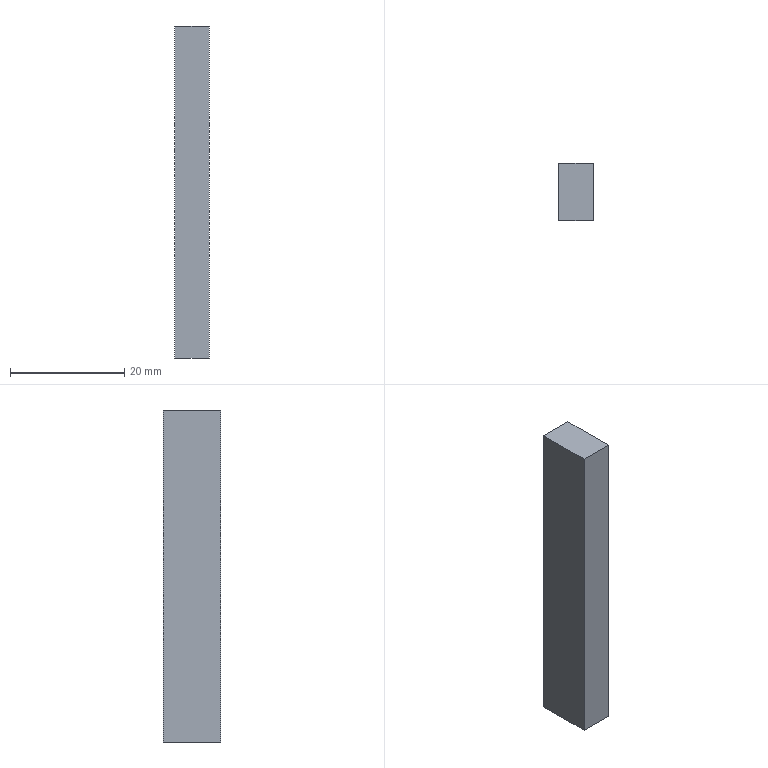Part | NX | features BREP 1 | 1 solid | 6 faces | box 6 x 10 x 58.1 mm | volume 3486 mm3 | plane 6
STEP:
#1=CARTESIAN_POINT('',(-1.25,10.55,-6.1));
#2=VERTEX_POINT('',#1);
#3=CARTESIAN_POINT('',(-1.25,0.55,-6.1));
#4=VERTEX_POINT('',#3);
#5=CARTESIAN_POINT('',(-1.25,10.55,-6.1));
#6=DIRECTION('',(0.,-1.,0.));
#7=VECTOR('',#6,1000.);
#8=LINE('',#5,#7);
#9=EDGE_CURVE('',#2,#4,#8,.T.);
#10=ORIENTED_EDGE('',*,*,#9,.T.);
#11=CARTESIAN_POINT('',(-1.25,0.55,52.));
#12=VERTEX_POINT('',#11);
#13=CARTESIAN_POINT('',(-1.25,0.55,52.));
#14=DIRECTION('',(0.,0.,-1.));
#15=VECTOR('',#14,1000.);
#16=LINE('',#13,#15);
#17=EDGE_CURVE('',#12,#4,#16,.T.);
#18=ORIENTED_EDGE('',*,*,#17,.F.);
#19=CARTESIAN_POINT('',(-1.25,10.55,52.));
#20=VERTEX_POINT('',#19);
#21=CARTESIAN_POINT('',(-1.25,10.55,52.));
#22=DIRECTION('',(0.,-1.,0.));
#23=VECTOR('',#22,1000.);
#24=LINE('',#21,#23);
#25=EDGE_CURVE('',#20,#12,#24,.T.);
#26=ORIENTED_EDGE('',*,*,#25,.F.);
#27=CARTESIAN_POINT('',(-1.25,10.55,52.));
#28=DIRECTION('',(0.,0.,-1.));
#29=VECTOR('',#28,1000.);
#30=LINE('',#27,#29);
#31=EDGE_CURVE('',#20,#2,#30,.T.);
#32=ORIENTED_EDGE('',*,*,#31,.T.);
#33=EDGE_LOOP('',(#10,#18,#26,#32));
#34=FACE_BOUND('',#33,.T.);
#35=CARTESIAN_POINT('',(-1.25,10.55,52.));
#36=DIRECTION('',(1.,0.,0.));
#37=DIRECTION('',(0.,0.,1.));
#38=AXIS2_PLACEMENT_3D('',#35,#36,#37);
#39=PLANE('',#38);
#40=ADVANCED_FACE('',(#34),#39,.F.);
#41=CARTESIAN_POINT('',(4.75,0.55,-6.1));
#42=VERTEX_POINT('',#41);
#43=CARTESIAN_POINT('',(-1.25,0.55,-6.1));
#44=DIRECTION('',(1.,0.,0.));
#45=VECTOR('',#44,1000.);
#46=LINE('',#43,#45);
#47=EDGE_CURVE('',#4,#42,#46,.T.);
#48=ORIENTED_EDGE('',*,*,#47,.T.);
#49=CARTESIAN_POINT('',(4.75,0.55,52.));
#50=VERTEX_POINT('',#49);
#51=CARTESIAN_POINT('',(4.75,0.55,52.));
#52=DIRECTION('',(0.,0.,-1.));
#53=VECTOR('',#52,1000.);
#54=LINE('',#51,#53);
#55=EDGE_CURVE('',#50,#42,#54,.T.);
#56=ORIENTED_EDGE('',*,*,#55,.F.);
#57=CARTESIAN_POINT('',(-1.25,0.55,52.));
#58=DIRECTION('',(1.,0.,0.));
#59=VECTOR('',#58,1000.);
#60=LINE('',#57,#59);
#61=EDGE_CURVE('',#12,#50,#60,.T.);
#62=ORIENTED_EDGE('',*,*,#61,.F.);
#63=ORIENTED_EDGE('',*,*,#17,.T.);
#64=EDGE_LOOP('',(#48,#56,#62,#63));
#65=FACE_BOUND('',#64,.T.);
#66=CARTESIAN_POINT('',(-1.25,0.55,52.));
#67=DIRECTION('',(0.,1.,0.));
#68=DIRECTION('',(0.,0.,-1.));
#69=AXIS2_PLACEMENT_3D('',#66,#67,#68);
#70=PLANE('',#69);
#71=ADVANCED_FACE('',(#65),#70,.F.);
#72=CARTESIAN_POINT('',(4.75,10.55,-6.1));
#73=VERTEX_POINT('',#72);
#74=CARTESIAN_POINT('',(4.75,0.55,-6.1));
#75=DIRECTION('',(0.,1.,0.));
#76=VECTOR('',#75,1000.);
#77=LINE('',#74,#76);
#78=EDGE_CURVE('',#42,#73,#77,.T.);
#79=ORIENTED_EDGE('',*,*,#78,.T.);
#80=CARTESIAN_POINT('',(4.75,10.55,52.));
#81=VERTEX_POINT('',#80);
#82=CARTESIAN_POINT('',(4.75,10.55,52.));
#83=DIRECTION('',(0.,0.,-1.));
#84=VECTOR('',#83,1000.);
#85=LINE('',#82,#84);
#86=EDGE_CURVE('',#81,#73,#85,.T.);
#87=ORIENTED_EDGE('',*,*,#86,.F.);
#88=CARTESIAN_POINT('',(4.75,0.55,52.));
#89=DIRECTION('',(0.,1.,0.));
#90=VECTOR('',#89,1000.);
#91=LINE('',#88,#90);
#92=EDGE_CURVE('',#50,#81,#91,.T.);
#93=ORIENTED_EDGE('',*,*,#92,.F.);
#94=ORIENTED_EDGE('',*,*,#55,.T.);
#95=EDGE_LOOP('',(#79,#87,#93,#94));
#96=FACE_BOUND('',#95,.T.);
#97=CARTESIAN_POINT('',(4.75,0.55,52.));
#98=DIRECTION('',(-1.,0.,0.));
#99=DIRECTION('',(0.,0.,-1.));
#100=AXIS2_PLACEMENT_3D('',#97,#98,#99);
#101=PLANE('',#100);
#102=ADVANCED_FACE('',(#96),#101,.F.);
#103=CARTESIAN_POINT('',(4.75,10.55,-6.1));
#104=DIRECTION('',(-1.,0.,0.));
#105=VECTOR('',#104,1000.);
#106=LINE('',#103,#105);
#107=EDGE_CURVE('',#73,#2,#106,.T.);
#108=ORIENTED_EDGE('',*,*,#107,.T.);
#109=ORIENTED_EDGE('',*,*,#31,.F.);
#110=CARTESIAN_POINT('',(4.75,10.55,52.));
#111=DIRECTION('',(-1.,0.,0.));
#112=VECTOR('',#111,1000.);
#113=LINE('',#110,#112);
#114=EDGE_CURVE('',#81,#20,#113,.T.);
#115=ORIENTED_EDGE('',*,*,#114,.F.);
#116=ORIENTED_EDGE('',*,*,#86,.T.);
#117=EDGE_LOOP('',(#108,#109,#115,#116));
#118=FACE_BOUND('',#117,.T.);
#119=CARTESIAN_POINT('',(4.75,10.55,52.));
#120=DIRECTION('',(0.,-1.,0.));
#121=DIRECTION('',(0.,0.,1.));
#122=AXIS2_PLACEMENT_3D('',#119,#120,#121);
#123=PLANE('',#122);
#124=ADVANCED_FACE('',(#118),#123,.F.);
#125=ORIENTED_EDGE('',*,*,#25,.T.);
#126=ORIENTED_EDGE('',*,*,#61,.T.);
#127=ORIENTED_EDGE('',*,*,#92,.T.);
#128=ORIENTED_EDGE('',*,*,#114,.T.);
#129=EDGE_LOOP('',(#125,#126,#127,#128));
#130=FACE_BOUND('',#129,.T.);
#131=CARTESIAN_POINT('',(0.,0.,52.));
#132=DIRECTION('',(0.,0.,1.));
#133=DIRECTION('',(-1.,0.,0.));
#134=AXIS2_PLACEMENT_3D('',#131,#132,#133);
#135=PLANE('',#134);
#136=ADVANCED_FACE('',(#130),#135,.T.);
#137=ORIENTED_EDGE('',*,*,#9,.F.);
#138=ORIENTED_EDGE('',*,*,#107,.F.);
#139=ORIENTED_EDGE('',*,*,#78,.F.);
#140=ORIENTED_EDGE('',*,*,#47,.F.);
#141=EDGE_LOOP('',(#137,#138,#139,#140));
#142=FACE_BOUND('',#141,.T.);
#143=CARTESIAN_POINT('',(0.,0.,-6.1));
#144=DIRECTION('',(0.,0.,1.));
#145=DIRECTION('',(-1.,0.,0.));
#146=AXIS2_PLACEMENT_3D('',#143,#144,#145);
#147=PLANE('',#146);
#148=ADVANCED_FACE('',(#142),#147,.F.);
#149=CLOSED_SHELL('',(#40,#71,#102,#124,#136,#148));
#150=MANIFOLD_SOLID_BREP('',#149);
#151=(LENGTH_UNIT()NAMED_UNIT(*)SI_UNIT(.MILLI.,.METRE.));
#152=UNCERTAINTY_MEASURE_WITH_UNIT(LENGTH_MEASURE(0.00001),#151,'','');
#153=(NAMED_UNIT(*)PLANE_ANGLE_UNIT()SI_UNIT($,.RADIAN.));
#154=(NAMED_UNIT(*)SI_UNIT($,.STERADIAN.)SOLID_ANGLE_UNIT());
#155=(GEOMETRIC_REPRESENTATION_CONTEXT(3)GLOBAL_UNCERTAINTY_ASSIGNED_CONTEXT((#152))GLOBAL_UNIT_ASSIGNED_CONTEXT((#151,#153,#154))REPRESENTATION_CONTEXT('',''));
#156=ADVANCED_BREP_SHAPE_REPRESENTATION('',(#150),#155);